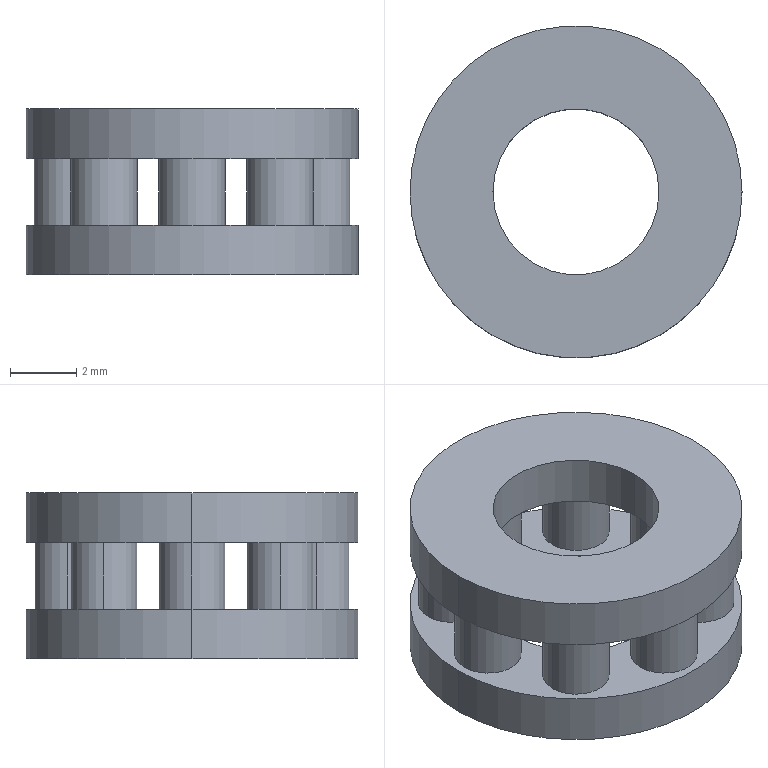Part | SolidWorks | features ICE 2, Extrusion 1 | 1 solid | 28 faces | box 10 x 10 x 5 mm | volume 226.98 mm3 | cylinder 24 | plane 4 | commonest cylinder face diameters 2 x16 5 x4 10 x4
STEP:
#1=CARTESIAN_POINT('',(-3.652,2.652,1.));
#2=VERTEX_POINT('',#1);
#3=CARTESIAN_POINT('',(-1.652,2.652,1.));
#4=VERTEX_POINT('',#3);
#5=CARTESIAN_POINT('',(-2.652,2.652,1.));
#6=DIRECTION('',(0.,0.,-1.));
#7=DIRECTION('',(1.,0.,0.));
#8=AXIS2_PLACEMENT_3D('',#5,#6,#7);
#9=CIRCLE('',#8,1.);
#10=EDGE_CURVE('',#2,#4,#9,.T.);
#11=ORIENTED_EDGE('',*,*,#10,.T.);
#12=CARTESIAN_POINT('',(-1.652,2.652,-1.));
#13=VERTEX_POINT('',#12);
#14=CARTESIAN_POINT('',(-1.652,2.652,1.));
#15=DIRECTION('',(0.,0.,-1.));
#16=VECTOR('',#15,1000.);
#17=LINE('',#14,#16);
#18=EDGE_CURVE('',#4,#13,#17,.T.);
#19=ORIENTED_EDGE('',*,*,#18,.T.);
#20=CARTESIAN_POINT('',(-3.652,2.652,-1.));
#21=VERTEX_POINT('',#20);
#22=CARTESIAN_POINT('',(-2.652,2.652,-1.));
#23=DIRECTION('',(0.,0.,1.));
#24=DIRECTION('',(1.,0.,0.));
#25=AXIS2_PLACEMENT_3D('',#22,#23,#24);
#26=CIRCLE('',#25,1.);
#27=EDGE_CURVE('',#13,#21,#26,.T.);
#28=ORIENTED_EDGE('',*,*,#27,.T.);
#29=CARTESIAN_POINT('',(-3.652,2.652,1.));
#30=DIRECTION('',(0.,0.,-1.));
#31=VECTOR('',#30,1000.);
#32=LINE('',#29,#31);
#33=EDGE_CURVE('',#2,#21,#32,.T.);
#34=ORIENTED_EDGE('',*,*,#33,.F.);
#35=EDGE_LOOP('',(#11,#19,#28,#34));
#36=FACE_OUTER_BOUND('',#35,.T.);
#37=CARTESIAN_POINT('',(-2.652,2.652,1.));
#38=DIRECTION('',(0.,0.,-1.));
#39=DIRECTION('',(-1.,0.,0.));
#40=AXIS2_PLACEMENT_3D('',#37,#38,#39);
#41=CYLINDRICAL_SURFACE('',#40,1.);
#42=ADVANCED_FACE('',(#36),#41,.T.);
#43=CARTESIAN_POINT('',(-4.75,0.,1.));
#44=VERTEX_POINT('',#43);
#45=CARTESIAN_POINT('',(-2.75,0.,1.));
#46=VERTEX_POINT('',#45);
#47=CARTESIAN_POINT('',(-3.75,0.,1.));
#48=DIRECTION('',(0.,0.,-1.));
#49=DIRECTION('',(1.,0.,0.));
#50=AXIS2_PLACEMENT_3D('',#47,#48,#49);
#51=CIRCLE('',#50,1.);
#52=EDGE_CURVE('',#44,#46,#51,.T.);
#53=ORIENTED_EDGE('',*,*,#52,.T.);
#54=CARTESIAN_POINT('',(-2.75,0.,-1.));
#55=VERTEX_POINT('',#54);
#56=CARTESIAN_POINT('',(-2.75,0.,1.));
#57=DIRECTION('',(0.,0.,-1.));
#58=VECTOR('',#57,1000.);
#59=LINE('',#56,#58);
#60=EDGE_CURVE('',#46,#55,#59,.T.);
#61=ORIENTED_EDGE('',*,*,#60,.T.);
#62=CARTESIAN_POINT('',(-4.75,0.,-1.));
#63=VERTEX_POINT('',#62);
#64=CARTESIAN_POINT('',(-3.75,0.,-1.));
#65=DIRECTION('',(0.,0.,1.));
#66=DIRECTION('',(1.,0.,0.));
#67=AXIS2_PLACEMENT_3D('',#64,#65,#66);
#68=CIRCLE('',#67,1.);
#69=EDGE_CURVE('',#55,#63,#68,.T.);
#70=ORIENTED_EDGE('',*,*,#69,.T.);
#71=CARTESIAN_POINT('',(-4.75,0.,1.));
#72=DIRECTION('',(0.,0.,-1.));
#73=VECTOR('',#72,1000.);
#74=LINE('',#71,#73);
#75=EDGE_CURVE('',#44,#63,#74,.T.);
#76=ORIENTED_EDGE('',*,*,#75,.F.);
#77=EDGE_LOOP('',(#53,#61,#70,#76));
#78=FACE_OUTER_BOUND('',#77,.T.);
#79=CARTESIAN_POINT('',(-3.75,0.,1.));
#80=DIRECTION('',(0.,0.,-1.));
#81=DIRECTION('',(-1.,0.,0.));
#82=AXIS2_PLACEMENT_3D('',#79,#80,#81);
#83=CYLINDRICAL_SURFACE('',#82,1.);
#84=ADVANCED_FACE('',(#78),#83,.T.);
#85=CARTESIAN_POINT('',(-3.652,-2.652,1.));
#86=VERTEX_POINT('',#85);
#87=CARTESIAN_POINT('',(-1.652,-2.652,1.));
#88=VERTEX_POINT('',#87);
#89=CARTESIAN_POINT('',(-2.652,-2.652,1.));
#90=DIRECTION('',(0.,0.,-1.));
#91=DIRECTION('',(1.,0.,0.));
#92=AXIS2_PLACEMENT_3D('',#89,#90,#91);
#93=CIRCLE('',#92,1.);
#94=EDGE_CURVE('',#86,#88,#93,.T.);
#95=ORIENTED_EDGE('',*,*,#94,.T.);
#96=CARTESIAN_POINT('',(-1.652,-2.652,-1.));
#97=VERTEX_POINT('',#96);
#98=CARTESIAN_POINT('',(-1.652,-2.652,1.));
#99=DIRECTION('',(0.,0.,-1.));
#100=VECTOR('',#99,1000.);
#101=LINE('',#98,#100);
#102=EDGE_CURVE('',#88,#97,#101,.T.);
#103=ORIENTED_EDGE('',*,*,#102,.T.);
#104=CARTESIAN_POINT('',(-3.652,-2.652,-1.));
#105=VERTEX_POINT('',#104);
#106=CARTESIAN_POINT('',(-2.652,-2.652,-1.));
#107=DIRECTION('',(0.,0.,1.));
#108=DIRECTION('',(1.,0.,0.));
#109=AXIS2_PLACEMENT_3D('',#106,#107,#108);
#110=CIRCLE('',#109,1.);
#111=EDGE_CURVE('',#97,#105,#110,.T.);
#112=ORIENTED_EDGE('',*,*,#111,.T.);
#113=CARTESIAN_POINT('',(-3.652,-2.652,1.));
#114=DIRECTION('',(0.,0.,-1.));
#115=VECTOR('',#114,1000.);
#116=LINE('',#113,#115);
#117=EDGE_CURVE('',#86,#105,#116,.T.);
#118=ORIENTED_EDGE('',*,*,#117,.F.);
#119=EDGE_LOOP('',(#95,#103,#112,#118));
#120=FACE_OUTER_BOUND('',#119,.T.);
#121=CARTESIAN_POINT('',(-2.652,-2.652,1.));
#122=DIRECTION('',(0.,0.,-1.));
#123=DIRECTION('',(-1.,0.,0.));
#124=AXIS2_PLACEMENT_3D('',#121,#122,#123);
#125=CYLINDRICAL_SURFACE('',#124,1.);
#126=ADVANCED_FACE('',(#120),#125,.T.);
#127=CARTESIAN_POINT('',(-1.,-3.75,1.));
#128=VERTEX_POINT('',#127);
#129=CARTESIAN_POINT('',(1.,-3.75,1.));
#130=VERTEX_POINT('',#129);
#131=CARTESIAN_POINT('',(0.,-3.75,1.));
#132=DIRECTION('',(0.,0.,-1.));
#133=DIRECTION('',(1.,0.,0.));
#134=AXIS2_PLACEMENT_3D('',#131,#132,#133);
#135=CIRCLE('',#134,1.);
#136=EDGE_CURVE('',#128,#130,#135,.T.);
#137=ORIENTED_EDGE('',*,*,#136,.T.);
#138=CARTESIAN_POINT('',(1.,-3.75,-1.));
#139=VERTEX_POINT('',#138);
#140=CARTESIAN_POINT('',(1.,-3.75,1.));
#141=DIRECTION('',(0.,0.,-1.));
#142=VECTOR('',#141,1000.);
#143=LINE('',#140,#142);
#144=EDGE_CURVE('',#130,#139,#143,.T.);
#145=ORIENTED_EDGE('',*,*,#144,.T.);
#146=CARTESIAN_POINT('',(-1.,-3.75,-1.));
#147=VERTEX_POINT('',#146);
#148=CARTESIAN_POINT('',(0.,-3.75,-1.));
#149=DIRECTION('',(0.,0.,1.));
#150=DIRECTION('',(1.,0.,0.));
#151=AXIS2_PLACEMENT_3D('',#148,#149,#150);
#152=CIRCLE('',#151,1.);
#153=EDGE_CURVE('',#139,#147,#152,.T.);
#154=ORIENTED_EDGE('',*,*,#153,.T.);
#155=CARTESIAN_POINT('',(-1.,-3.75,1.));
#156=DIRECTION('',(0.,0.,-1.));
#157=VECTOR('',#156,1000.);
#158=LINE('',#155,#157);
#159=EDGE_CURVE('',#128,#147,#158,.T.);
#160=ORIENTED_EDGE('',*,*,#159,.F.);
#161=EDGE_LOOP('',(#137,#145,#154,#160));
#162=FACE_OUTER_BOUND('',#161,.T.);
#163=CARTESIAN_POINT('',(0.,-3.75,1.));
#164=DIRECTION('',(0.,0.,-1.));
#165=DIRECTION('',(-1.,0.,0.));
#166=AXIS2_PLACEMENT_3D('',#163,#164,#165);
#167=CYLINDRICAL_SURFACE('',#166,1.);
#168=ADVANCED_FACE('',(#162),#167,.T.);
#169=CARTESIAN_POINT('',(1.652,-2.652,1.));
#170=VERTEX_POINT('',#169);
#171=CARTESIAN_POINT('',(3.652,-2.652,1.));
#172=VERTEX_POINT('',#171);
#173=CARTESIAN_POINT('',(2.652,-2.652,1.));
#174=DIRECTION('',(0.,0.,-1.));
#175=DIRECTION('',(1.,0.,0.));
#176=AXIS2_PLACEMENT_3D('',#173,#174,#175);
#177=CIRCLE('',#176,1.);
#178=EDGE_CURVE('',#170,#172,#177,.T.);
#179=ORIENTED_EDGE('',*,*,#178,.T.);
#180=CARTESIAN_POINT('',(3.652,-2.652,-1.));
#181=VERTEX_POINT('',#180);
#182=CARTESIAN_POINT('',(3.652,-2.652,1.));
#183=DIRECTION('',(0.,0.,-1.));
#184=VECTOR('',#183,1000.);
#185=LINE('',#182,#184);
#186=EDGE_CURVE('',#172,#181,#185,.T.);
#187=ORIENTED_EDGE('',*,*,#186,.T.);
#188=CARTESIAN_POINT('',(1.652,-2.652,-1.));
#189=VERTEX_POINT('',#188);
#190=CARTESIAN_POINT('',(2.652,-2.652,-1.));
#191=DIRECTION('',(0.,0.,1.));
#192=DIRECTION('',(1.,0.,0.));
#193=AXIS2_PLACEMENT_3D('',#190,#191,#192);
#194=CIRCLE('',#193,1.);
#195=EDGE_CURVE('',#181,#189,#194,.T.);
#196=ORIENTED_EDGE('',*,*,#195,.T.);
#197=CARTESIAN_POINT('',(1.652,-2.652,1.));
#198=DIRECTION('',(0.,0.,-1.));
#199=VECTOR('',#198,1000.);
#200=LINE('',#197,#199);
#201=EDGE_CURVE('',#170,#189,#200,.T.);
#202=ORIENTED_EDGE('',*,*,#201,.F.);
#203=EDGE_LOOP('',(#179,#187,#196,#202));
#204=FACE_OUTER_BOUND('',#203,.T.);
#205=CARTESIAN_POINT('',(2.652,-2.652,1.));
#206=DIRECTION('',(0.,0.,-1.));
#207=DIRECTION('',(-1.,0.,0.));
#208=AXIS2_PLACEMENT_3D('',#205,#206,#207);
#209=CYLINDRICAL_SURFACE('',#208,1.);
#210=ADVANCED_FACE('',(#204),#209,.T.);
#211=CARTESIAN_POINT('',(2.75,0.,1.));
#212=VERTEX_POINT('',#211);
#213=CARTESIAN_POINT('',(4.75,0.,1.));
#214=VERTEX_POINT('',#213);
#215=CARTESIAN_POINT('',(3.75,0.,1.));
#216=DIRECTION('',(0.,0.,-1.));
#217=DIRECTION('',(1.,0.,0.));
#218=AXIS2_PLACEMENT_3D('',#215,#216,#217);
#219=CIRCLE('',#218,1.);
#220=EDGE_CURVE('',#212,#214,#219,.T.);
#221=ORIENTED_EDGE('',*,*,#220,.T.);
#222=CARTESIAN_POINT('',(4.75,0.,-1.));
#223=VERTEX_POINT('',#222);
#224=CARTESIAN_POINT('',(4.75,0.,1.));
#225=DIRECTION('',(0.,0.,-1.));
#226=VECTOR('',#225,1000.);
#227=LINE('',#224,#226);
#228=EDGE_CURVE('',#214,#223,#227,.T.);
#229=ORIENTED_EDGE('',*,*,#228,.T.);
#230=CARTESIAN_POINT('',(2.75,0.,-1.));
#231=VERTEX_POINT('',#230);
#232=CARTESIAN_POINT('',(3.75,0.,-1.));
#233=DIRECTION('',(0.,0.,1.));
#234=DIRECTION('',(1.,0.,0.));
#235=AXIS2_PLACEMENT_3D('',#232,#233,#234);
#236=CIRCLE('',#235,1.);
#237=EDGE_CURVE('',#223,#231,#236,.T.);
#238=ORIENTED_EDGE('',*,*,#237,.T.);
#239=CARTESIAN_POINT('',(2.75,0.,1.));
#240=DIRECTION('',(0.,0.,-1.));
#241=VECTOR('',#240,1000.);
#242=LINE('',#239,#241);
#243=EDGE_CURVE('',#212,#231,#242,.T.);
#244=ORIENTED_EDGE('',*,*,#243,.F.);
#245=EDGE_LOOP('',(#221,#229,#238,#244));
#246=FACE_OUTER_BOUND('',#245,.T.);
#247=CARTESIAN_POINT('',(3.75,0.,1.));
#248=DIRECTION('',(0.,0.,-1.));
#249=DIRECTION('',(-1.,0.,0.));
#250=AXIS2_PLACEMENT_3D('',#247,#248,#249);
#251=CYLINDRICAL_SURFACE('',#250,1.);
#252=ADVANCED_FACE('',(#246),#251,.T.);
#253=CARTESIAN_POINT('',(1.652,2.652,1.));
#254=VERTEX_POINT('',#253);
#255=CARTESIAN_POINT('',(3.652,2.652,1.));
#256=VERTEX_POINT('',#255);
#257=CARTESIAN_POINT('',(2.652,2.652,1.));
#258=DIRECTION('',(0.,0.,-1.));
#259=DIRECTION('',(1.,0.,0.));
#260=AXIS2_PLACEMENT_3D('',#257,#258,#259);
#261=CIRCLE('',#260,1.);
#262=EDGE_CURVE('',#254,#256,#261,.T.);
#263=ORIENTED_EDGE('',*,*,#262,.T.);
#264=CARTESIAN_POINT('',(3.652,2.652,-1.));
#265=VERTEX_POINT('',#264);
#266=CARTESIAN_POINT('',(3.652,2.652,1.));
#267=DIRECTION('',(0.,0.,-1.));
#268=VECTOR('',#267,1000.);
#269=LINE('',#266,#268);
#270=EDGE_CURVE('',#256,#265,#269,.T.);
#271=ORIENTED_EDGE('',*,*,#270,.T.);
#272=CARTESIAN_POINT('',(1.652,2.652,-1.));
#273=VERTEX_POINT('',#272);
#274=CARTESIAN_POINT('',(2.652,2.652,-1.));
#275=DIRECTION('',(0.,0.,1.));
#276=DIRECTION('',(1.,0.,0.));
#277=AXIS2_PLACEMENT_3D('',#274,#275,#276);
#278=CIRCLE('',#277,1.);
#279=EDGE_CURVE('',#265,#273,#278,.T.);
#280=ORIENTED_EDGE('',*,*,#279,.T.);
#281=CARTESIAN_POINT('',(1.652,2.652,1.));
#282=DIRECTION('',(0.,0.,-1.));
#283=VECTOR('',#282,1000.);
#284=LINE('',#281,#283);
#285=EDGE_CURVE('',#254,#273,#284,.T.);
#286=ORIENTED_EDGE('',*,*,#285,.F.);
#287=EDGE_LOOP('',(#263,#271,#280,#286));
#288=FACE_OUTER_BOUND('',#287,.T.);
#289=CARTESIAN_POINT('',(2.652,2.652,1.));
#290=DIRECTION('',(0.,0.,-1.));
#291=DIRECTION('',(-1.,0.,0.));
#292=AXIS2_PLACEMENT_3D('',#289,#290,#291);
#293=CYLINDRICAL_SURFACE('',#292,1.);
#294=ADVANCED_FACE('',(#288),#293,.T.);
#295=CARTESIAN_POINT('',(-2.5,0.,-2.5));
#296=VERTEX_POINT('',#295);
#297=CARTESIAN_POINT('',(2.5,0.,-2.5));
#298=VERTEX_POINT('',#297);
#299=CARTESIAN_POINT('',(0.,0.,-2.5));
#300=DIRECTION('',(0.,0.,1.));
#301=DIRECTION('',(1.,0.,0.));
#302=AXIS2_PLACEMENT_3D('',#299,#300,#301);
#303=CIRCLE('',#302,2.5);
#304=EDGE_CURVE('',#296,#298,#303,.T.);
#305=ORIENTED_EDGE('',*,*,#304,.F.);
#306=CARTESIAN_POINT('',(-2.5,0.,-1.));
#307=VERTEX_POINT('',#306);
#308=CARTESIAN_POINT('',(-2.5,0.,-2.5));
#309=DIRECTION('',(0.,0.,1.));
#310=VECTOR('',#309,1000.);
#311=LINE('',#308,#310);
#312=EDGE_CURVE('',#296,#307,#311,.T.);
#313=ORIENTED_EDGE('',*,*,#312,.T.);
#314=CARTESIAN_POINT('',(2.5,0.,-1.));
#315=VERTEX_POINT('',#314);
#316=CARTESIAN_POINT('',(0.,0.,-1.));
#317=DIRECTION('',(0.,0.,1.));
#318=DIRECTION('',(1.,0.,0.));
#319=AXIS2_PLACEMENT_3D('',#316,#317,#318);
#320=CIRCLE('',#319,2.5);
#321=EDGE_CURVE('',#307,#315,#320,.T.);
#322=ORIENTED_EDGE('',*,*,#321,.T.);
#323=CARTESIAN_POINT('',(2.5,0.,-2.5));
#324=DIRECTION('',(0.,0.,1.));
#325=VECTOR('',#324,1000.);
#326=LINE('',#323,#325);
#327=EDGE_CURVE('',#298,#315,#326,.T.);
#328=ORIENTED_EDGE('',*,*,#327,.F.);
#329=EDGE_LOOP('',(#305,#313,#322,#328));
#330=FACE_OUTER_BOUND('',#329,.T.);
#331=CARTESIAN_POINT('',(0.,0.,-2.5));
#332=DIRECTION('',(0.,0.,1.));
#333=DIRECTION('',(1.,0.,0.));
#334=AXIS2_PLACEMENT_3D('',#331,#332,#333);
#335=CYLINDRICAL_SURFACE('',#334,2.5);
#336=ADVANCED_FACE('',(#330),#335,.F.);
#337=CARTESIAN_POINT('',(5.,0.,-2.5));
#338=VERTEX_POINT('',#337);
#339=CARTESIAN_POINT('',(-5.,0.,-2.5));
#340=VERTEX_POINT('',#339);
#341=CARTESIAN_POINT('',(0.,0.,-2.5));
#342=DIRECTION('',(0.,0.,1.));
#343=DIRECTION('',(1.,0.,0.));
#344=AXIS2_PLACEMENT_3D('',#341,#342,#343);
#345=CIRCLE('',#344,5.);
#346=EDGE_CURVE('',#338,#340,#345,.T.);
#347=ORIENTED_EDGE('',*,*,#346,.T.);
#348=CARTESIAN_POINT('',(-5.,0.,-1.));
#349=VERTEX_POINT('',#348);
#350=CARTESIAN_POINT('',(-5.,0.,-2.5));
#351=DIRECTION('',(0.,0.,1.));
#352=VECTOR('',#351,1000.);
#353=LINE('',#350,#352);
#354=EDGE_CURVE('',#340,#349,#353,.T.);
#355=ORIENTED_EDGE('',*,*,#354,.T.);
#356=CARTESIAN_POINT('',(5.,0.,-1.));
#357=VERTEX_POINT('',#356);
#358=CARTESIAN_POINT('',(0.,0.,-1.));
#359=DIRECTION('',(0.,0.,1.));
#360=DIRECTION('',(1.,0.,0.));
#361=AXIS2_PLACEMENT_3D('',#358,#359,#360);
#362=CIRCLE('',#361,5.);
#363=EDGE_CURVE('',#357,#349,#362,.T.);
#364=ORIENTED_EDGE('',*,*,#363,.F.);
#365=CARTESIAN_POINT('',(5.,0.,-2.5));
#366=DIRECTION('',(0.,0.,1.));
#367=VECTOR('',#366,1000.);
#368=LINE('',#365,#367);
#369=EDGE_CURVE('',#338,#357,#368,.T.);
#370=ORIENTED_EDGE('',*,*,#369,.F.);
#371=EDGE_LOOP('',(#347,#355,#364,#370));
#372=FACE_OUTER_BOUND('',#371,.T.);
#373=CARTESIAN_POINT('',(0.,0.,-2.5));
#374=DIRECTION('',(0.,0.,1.));
#375=DIRECTION('',(1.,0.,0.));
#376=AXIS2_PLACEMENT_3D('',#373,#374,#375);
#377=CYLINDRICAL_SURFACE('',#376,5.);
#378=ADVANCED_FACE('',(#372),#377,.T.);
#379=CARTESIAN_POINT('',(-1.,3.75,1.));
#380=VERTEX_POINT('',#379);
#381=CARTESIAN_POINT('',(1.,3.75,1.));
#382=VERTEX_POINT('',#381);
#383=CARTESIAN_POINT('',(0.,3.75,1.));
#384=DIRECTION('',(0.,0.,-1.));
#385=DIRECTION('',(1.,0.,0.));
#386=AXIS2_PLACEMENT_3D('',#383,#384,#385);
#387=CIRCLE('',#386,1.);
#388=EDGE_CURVE('',#380,#382,#387,.T.);
#389=ORIENTED_EDGE('',*,*,#388,.T.);
#390=CARTESIAN_POINT('',(1.,3.75,-1.));
#391=VERTEX_POINT('',#390);
#392=CARTESIAN_POINT('',(1.,3.75,1.));
#393=DIRECTION('',(0.,0.,-1.));
#394=VECTOR('',#393,1000.);
#395=LINE('',#392,#394);
#396=EDGE_CURVE('',#382,#391,#395,.T.);
#397=ORIENTED_EDGE('',*,*,#396,.T.);
#398=CARTESIAN_POINT('',(-1.,3.75,-1.));
#399=VERTEX_POINT('',#398);
#400=CARTESIAN_POINT('',(0.,3.75,-1.));
#401=DIRECTION('',(0.,0.,1.));
#402=DIRECTION('',(1.,0.,0.));
#403=AXIS2_PLACEMENT_3D('',#400,#401,#402);
#404=CIRCLE('',#403,1.);
#405=EDGE_CURVE('',#391,#399,#404,.T.);
#406=ORIENTED_EDGE('',*,*,#405,.T.);
#407=CARTESIAN_POINT('',(-1.,3.75,1.));
#408=DIRECTION('',(0.,0.,-1.));
#409=VECTOR('',#408,1000.);
#410=LINE('',#407,#409);
#411=EDGE_CURVE('',#380,#399,#410,.T.);
#412=ORIENTED_EDGE('',*,*,#411,.F.);
#413=EDGE_LOOP('',(#389,#397,#406,#412));
#414=FACE_OUTER_BOUND('',#413,.T.);
#415=CARTESIAN_POINT('',(0.,3.75,1.));
#416=DIRECTION('',(0.,0.,-1.));
#417=DIRECTION('',(-1.,0.,0.));
#418=AXIS2_PLACEMENT_3D('',#415,#416,#417);
#419=CYLINDRICAL_SURFACE('',#418,1.);
#420=ADVANCED_FACE('',(#414),#419,.T.);
#421=CARTESIAN_POINT('',(-2.5,0.,2.5));
#422=VERTEX_POINT('',#421);
#423=CARTESIAN_POINT('',(2.5,0.,2.5));
#424=VERTEX_POINT('',#423);
#425=CARTESIAN_POINT('',(0.,0.,2.5));
#426=DIRECTION('',(0.,0.,1.));
#427=DIRECTION('',(1.,0.,0.));
#428=AXIS2_PLACEMENT_3D('',#425,#426,#427);
#429=CIRCLE('',#428,2.5);
#430=EDGE_CURVE('',#422,#424,#429,.T.);
#431=ORIENTED_EDGE('',*,*,#430,.T.);
#432=CARTESIAN_POINT('',(2.5,0.,1.));
#433=VERTEX_POINT('',#432);
#434=CARTESIAN_POINT('',(2.5,0.,2.5));
#435=DIRECTION('',(0.,0.,-1.));
#436=VECTOR('',#435,1000.);
#437=LINE('',#434,#436);
#438=EDGE_CURVE('',#424,#433,#437,.T.);
#439=ORIENTED_EDGE('',*,*,#438,.T.);
#440=CARTESIAN_POINT('',(-2.5,0.,1.));
#441=VERTEX_POINT('',#440);
#442=CARTESIAN_POINT('',(0.,0.,1.));
#443=DIRECTION('',(0.,0.,1.));
#444=DIRECTION('',(1.,0.,0.));
#445=AXIS2_PLACEMENT_3D('',#442,#443,#444);
#446=CIRCLE('',#445,2.5);
#447=EDGE_CURVE('',#441,#433,#446,.T.);
#448=ORIENTED_EDGE('',*,*,#447,.F.);
#449=CARTESIAN_POINT('',(-2.5,0.,2.5));
#450=DIRECTION('',(0.,0.,-1.));
#451=VECTOR('',#450,1000.);
#452=LINE('',#449,#451);
#453=EDGE_CURVE('',#422,#441,#452,.T.);
#454=ORIENTED_EDGE('',*,*,#453,.F.);
#455=EDGE_LOOP('',(#431,#439,#448,#454));
#456=FACE_OUTER_BOUND('',#455,.T.);
#457=CARTESIAN_POINT('',(0.,0.,2.5));
#458=DIRECTION('',(0.,0.,-1.));
#459=DIRECTION('',(-1.,0.,0.));
#460=AXIS2_PLACEMENT_3D('',#457,#458,#459);
#461=CYLINDRICAL_SURFACE('',#460,2.5);
#462=ADVANCED_FACE('',(#456),#461,.F.);
#463=CARTESIAN_POINT('',(5.,0.,2.5));
#464=VERTEX_POINT('',#463);
#465=CARTESIAN_POINT('',(-5.,0.,2.5));
#466=VERTEX_POINT('',#465);
#467=CARTESIAN_POINT('',(0.,0.,2.5));
#468=DIRECTION('',(0.,0.,1.));
#469=DIRECTION('',(1.,0.,0.));
#470=AXIS2_PLACEMENT_3D('',#467,#468,#469);
#471=CIRCLE('',#470,5.);
#472=EDGE_CURVE('',#464,#466,#471,.T.);
#473=ORIENTED_EDGE('',*,*,#472,.F.);
#474=CARTESIAN_POINT('',(5.,0.,1.));
#475=VERTEX_POINT('',#474);
#476=CARTESIAN_POINT('',(5.,0.,2.5));
#477=DIRECTION('',(0.,0.,-1.));
#478=VECTOR('',#477,1000.);
#479=LINE('',#476,#478);
#480=EDGE_CURVE('',#464,#475,#479,.T.);
#481=ORIENTED_EDGE('',*,*,#480,.T.);
#482=CARTESIAN_POINT('',(-5.,0.,1.));
#483=VERTEX_POINT('',#482);
#484=CARTESIAN_POINT('',(0.,0.,1.));
#485=DIRECTION('',(0.,0.,1.));
#486=DIRECTION('',(1.,0.,0.));
#487=AXIS2_PLACEMENT_3D('',#484,#485,#486);
#488=CIRCLE('',#487,5.);
#489=EDGE_CURVE('',#475,#483,#488,.T.);
#490=ORIENTED_EDGE('',*,*,#489,.T.);
#491=CARTESIAN_POINT('',(-5.,0.,2.5));
#492=DIRECTION('',(0.,0.,-1.));
#493=VECTOR('',#492,1000.);
#494=LINE('',#491,#493);
#495=EDGE_CURVE('',#466,#483,#494,.T.);
#496=ORIENTED_EDGE('',*,*,#495,.F.);
#497=EDGE_LOOP('',(#473,#481,#490,#496));
#498=FACE_OUTER_BOUND('',#497,.T.);
#499=CARTESIAN_POINT('',(0.,0.,2.5));
#500=DIRECTION('',(0.,0.,-1.));
#501=DIRECTION('',(-1.,0.,0.));
#502=AXIS2_PLACEMENT_3D('',#499,#500,#501);
#503=CYLINDRICAL_SURFACE('',#502,5.);
#504=ADVANCED_FACE('',(#498),#503,.T.);
#505=CARTESIAN_POINT('',(0.,0.,2.5));
#506=DIRECTION('',(0.,0.,1.));
#507=DIRECTION('',(1.,0.,0.));
#508=AXIS2_PLACEMENT_3D('',#505,#506,#507);
#509=CIRCLE('',#508,5.);
#510=EDGE_CURVE('',#466,#464,#509,.T.);
#511=ORIENTED_EDGE('',*,*,#510,.T.);
#512=ORIENTED_EDGE('',*,*,#472,.T.);
#513=EDGE_LOOP('',(#511,#512));
#514=FACE_OUTER_BOUND('',#513,.T.);
#515=ORIENTED_EDGE('',*,*,#430,.F.);
#516=CARTESIAN_POINT('',(0.,0.,2.5));
#517=DIRECTION('',(0.,0.,1.));
#518=DIRECTION('',(1.,0.,0.));
#519=AXIS2_PLACEMENT_3D('',#516,#517,#518);
#520=CIRCLE('',#519,2.5);
#521=EDGE_CURVE('',#424,#422,#520,.T.);
#522=ORIENTED_EDGE('',*,*,#521,.F.);
#523=EDGE_LOOP('',(#515,#522));
#524=FACE_BOUND('',#523,.T.);
#525=CARTESIAN_POINT('',(0.,0.,2.5));
#526=DIRECTION('',(0.,0.,1.));
#527=DIRECTION('',(1.,0.,0.));
#528=AXIS2_PLACEMENT_3D('',#525,#526,#527);
#529=PLANE('',#528);
#530=ADVANCED_FACE('',(#514,#524),#529,.T.);
#531=ORIENTED_EDGE('',*,*,#10,.F.);
#532=CARTESIAN_POINT('',(-2.652,2.652,1.));
#533=DIRECTION('',(0.,0.,-1.));
#534=DIRECTION('',(1.,0.,0.));
#535=AXIS2_PLACEMENT_3D('',#532,#533,#534);
#536=CIRCLE('',#535,1.);
#537=EDGE_CURVE('',#4,#2,#536,.T.);
#538=ORIENTED_EDGE('',*,*,#537,.F.);
#539=EDGE_LOOP('',(#531,#538));
#540=FACE_BOUND('',#539,.T.);
#541=ORIENTED_EDGE('',*,*,#52,.F.);
#542=CARTESIAN_POINT('',(-3.75,0.,1.));
#543=DIRECTION('',(0.,0.,-1.));
#544=DIRECTION('',(1.,0.,0.));
#545=AXIS2_PLACEMENT_3D('',#542,#543,#544);
#546=CIRCLE('',#545,1.);
#547=EDGE_CURVE('',#46,#44,#546,.T.);
#548=ORIENTED_EDGE('',*,*,#547,.F.);
#549=EDGE_LOOP('',(#541,#548));
#550=FACE_BOUND('',#549,.T.);
#551=ORIENTED_EDGE('',*,*,#94,.F.);
#552=CARTESIAN_POINT('',(-2.652,-2.652,1.));
#553=DIRECTION('',(0.,0.,-1.));
#554=DIRECTION('',(1.,0.,0.));
#555=AXIS2_PLACEMENT_3D('',#552,#553,#554);
#556=CIRCLE('',#555,1.);
#557=EDGE_CURVE('',#88,#86,#556,.T.);
#558=ORIENTED_EDGE('',*,*,#557,.F.);
#559=EDGE_LOOP('',(#551,#558));
#560=FACE_BOUND('',#559,.T.);
#561=ORIENTED_EDGE('',*,*,#136,.F.);
#562=CARTESIAN_POINT('',(0.,-3.75,1.));
#563=DIRECTION('',(0.,0.,-1.));
#564=DIRECTION('',(1.,0.,0.));
#565=AXIS2_PLACEMENT_3D('',#562,#563,#564);
#566=CIRCLE('',#565,1.);
#567=EDGE_CURVE('',#130,#128,#566,.T.);
#568=ORIENTED_EDGE('',*,*,#567,.F.);
#569=EDGE_LOOP('',(#561,#568));
#570=FACE_BOUND('',#569,.T.);
#571=ORIENTED_EDGE('',*,*,#178,.F.);
#572=CARTESIAN_POINT('',(2.652,-2.652,1.));
#573=DIRECTION('',(0.,0.,-1.));
#574=DIRECTION('',(1.,0.,0.));
#575=AXIS2_PLACEMENT_3D('',#572,#573,#574);
#576=CIRCLE('',#575,1.);
#577=EDGE_CURVE('',#172,#170,#576,.T.);
#578=ORIENTED_EDGE('',*,*,#577,.F.);
#579=EDGE_LOOP('',(#571,#578));
#580=FACE_BOUND('',#579,.T.);
#581=ORIENTED_EDGE('',*,*,#220,.F.);
#582=CARTESIAN_POINT('',(3.75,0.,1.));
#583=DIRECTION('',(0.,0.,-1.));
#584=DIRECTION('',(1.,0.,0.));
#585=AXIS2_PLACEMENT_3D('',#582,#583,#584);
#586=CIRCLE('',#585,1.);
#587=EDGE_CURVE('',#214,#212,#586,.T.);
#588=ORIENTED_EDGE('',*,*,#587,.F.);
#589=EDGE_LOOP('',(#581,#588));
#590=FACE_BOUND('',#589,.T.);
#591=ORIENTED_EDGE('',*,*,#262,.F.);
#592=CARTESIAN_POINT('',(2.652,2.652,1.));
#593=DIRECTION('',(0.,0.,-1.));
#594=DIRECTION('',(1.,0.,0.));
#595=AXIS2_PLACEMENT_3D('',#592,#593,#594);
#596=CIRCLE('',#595,1.);
#597=EDGE_CURVE('',#256,#254,#596,.T.);
#598=ORIENTED_EDGE('',*,*,#597,.F.);
#599=EDGE_LOOP('',(#591,#598));
#600=FACE_BOUND('',#599,.T.);
#601=ORIENTED_EDGE('',*,*,#388,.F.);
#602=CARTESIAN_POINT('',(0.,3.75,1.));
#603=DIRECTION('',(0.,0.,-1.));
#604=DIRECTION('',(1.,0.,0.));
#605=AXIS2_PLACEMENT_3D('',#602,#603,#604);
#606=CIRCLE('',#605,1.);
#607=EDGE_CURVE('',#382,#380,#606,.T.);
#608=ORIENTED_EDGE('',*,*,#607,.F.);
#609=EDGE_LOOP('',(#601,#608));
#610=FACE_BOUND('',#609,.T.);
#611=CARTESIAN_POINT('',(0.,0.,1.));
#612=DIRECTION('',(0.,0.,1.));
#613=DIRECTION('',(1.,0.,0.));
#614=AXIS2_PLACEMENT_3D('',#611,#612,#613);
#615=CIRCLE('',#614,5.);
#616=EDGE_CURVE('',#483,#475,#615,.T.);
#617=ORIENTED_EDGE('',*,*,#616,.F.);
#618=ORIENTED_EDGE('',*,*,#489,.F.);
#619=EDGE_LOOP('',(#617,#618));
#620=FACE_OUTER_BOUND('',#619,.T.);
#621=ORIENTED_EDGE('',*,*,#447,.T.);
#622=CARTESIAN_POINT('',(0.,0.,1.));
#623=DIRECTION('',(0.,0.,1.));
#624=DIRECTION('',(1.,0.,0.));
#625=AXIS2_PLACEMENT_3D('',#622,#623,#624);
#626=CIRCLE('',#625,2.5);
#627=EDGE_CURVE('',#433,#441,#626,.T.);
#628=ORIENTED_EDGE('',*,*,#627,.T.);
#629=EDGE_LOOP('',(#621,#628));
#630=FACE_BOUND('',#629,.T.);
#631=CARTESIAN_POINT('',(0.,0.,1.));
#632=DIRECTION('',(0.,0.,1.));
#633=DIRECTION('',(1.,0.,0.));
#634=AXIS2_PLACEMENT_3D('',#631,#632,#633);
#635=PLANE('',#634);
#636=ADVANCED_FACE('',(#540,#550,#560,#570,#580,#590,#600,#610,#620,#630),#635,.F.);
#637=ORIENTED_EDGE('',*,*,#480,.F.);
#638=ORIENTED_EDGE('',*,*,#510,.F.);
#639=ORIENTED_EDGE('',*,*,#495,.T.);
#640=ORIENTED_EDGE('',*,*,#616,.T.);
#641=EDGE_LOOP('',(#637,#638,#639,#640));
#642=FACE_OUTER_BOUND('',#641,.T.);
#643=CARTESIAN_POINT('',(0.,0.,2.5));
#644=DIRECTION('',(0.,0.,-1.));
#645=DIRECTION('',(-1.,0.,0.));
#646=AXIS2_PLACEMENT_3D('',#643,#644,#645);
#647=CYLINDRICAL_SURFACE('',#646,5.);
#648=ADVANCED_FACE('',(#642),#647,.T.);
#649=ORIENTED_EDGE('',*,*,#438,.F.);
#650=ORIENTED_EDGE('',*,*,#521,.T.);
#651=ORIENTED_EDGE('',*,*,#453,.T.);
#652=ORIENTED_EDGE('',*,*,#627,.F.);
#653=EDGE_LOOP('',(#649,#650,#651,#652));
#654=FACE_OUTER_BOUND('',#653,.T.);
#655=CARTESIAN_POINT('',(0.,0.,2.5));
#656=DIRECTION('',(0.,0.,-1.));
#657=DIRECTION('',(-1.,0.,0.));
#658=AXIS2_PLACEMENT_3D('',#655,#656,#657);
#659=CYLINDRICAL_SURFACE('',#658,2.5);
#660=ADVANCED_FACE('',(#654),#659,.F.);
#661=ORIENTED_EDGE('',*,*,#396,.F.);
#662=ORIENTED_EDGE('',*,*,#607,.T.);
#663=ORIENTED_EDGE('',*,*,#411,.T.);
#664=CARTESIAN_POINT('',(0.,3.75,-1.));
#665=DIRECTION('',(0.,0.,1.));
#666=DIRECTION('',(1.,0.,0.));
#667=AXIS2_PLACEMENT_3D('',#664,#665,#666);
#668=CIRCLE('',#667,1.);
#669=EDGE_CURVE('',#399,#391,#668,.T.);
#670=ORIENTED_EDGE('',*,*,#669,.T.);
#671=EDGE_LOOP('',(#661,#662,#663,#670));
#672=FACE_OUTER_BOUND('',#671,.T.);
#673=CARTESIAN_POINT('',(0.,3.75,1.));
#674=DIRECTION('',(0.,0.,-1.));
#675=DIRECTION('',(-1.,0.,0.));
#676=AXIS2_PLACEMENT_3D('',#673,#674,#675);
#677=CYLINDRICAL_SURFACE('',#676,1.);
#678=ADVANCED_FACE('',(#672),#677,.T.);
#679=ORIENTED_EDGE('',*,*,#354,.F.);
#680=CARTESIAN_POINT('',(0.,0.,-2.5));
#681=DIRECTION('',(0.,0.,1.));
#682=DIRECTION('',(1.,0.,0.));
#683=AXIS2_PLACEMENT_3D('',#680,#681,#682);
#684=CIRCLE('',#683,5.);
#685=EDGE_CURVE('',#340,#338,#684,.T.);
#686=ORIENTED_EDGE('',*,*,#685,.T.);
#687=ORIENTED_EDGE('',*,*,#369,.T.);
#688=CARTESIAN_POINT('',(0.,0.,-1.));
#689=DIRECTION('',(0.,0.,1.));
#690=DIRECTION('',(1.,0.,0.));
#691=AXIS2_PLACEMENT_3D('',#688,#689,#690);
#692=CIRCLE('',#691,5.);
#693=EDGE_CURVE('',#349,#357,#692,.T.);
#694=ORIENTED_EDGE('',*,*,#693,.F.);
#695=EDGE_LOOP('',(#679,#686,#687,#694));
#696=FACE_OUTER_BOUND('',#695,.T.);
#697=CARTESIAN_POINT('',(0.,0.,-2.5));
#698=DIRECTION('',(0.,0.,1.));
#699=DIRECTION('',(1.,0.,0.));
#700=AXIS2_PLACEMENT_3D('',#697,#698,#699);
#701=CYLINDRICAL_SURFACE('',#700,5.);
#702=ADVANCED_FACE('',(#696),#701,.T.);
#703=CARTESIAN_POINT('',(0.,0.,-2.5));
#704=DIRECTION('',(0.,0.,1.));
#705=DIRECTION('',(1.,0.,0.));
#706=AXIS2_PLACEMENT_3D('',#703,#704,#705);
#707=CIRCLE('',#706,2.5);
#708=EDGE_CURVE('',#298,#296,#707,.T.);
#709=ORIENTED_EDGE('',*,*,#708,.T.);
#710=ORIENTED_EDGE('',*,*,#304,.T.);
#711=EDGE_LOOP('',(#709,#710));
#712=FACE_BOUND('',#711,.T.);
#713=ORIENTED_EDGE('',*,*,#346,.F.);
#714=ORIENTED_EDGE('',*,*,#685,.F.);
#715=EDGE_LOOP('',(#713,#714));
#716=FACE_OUTER_BOUND('',#715,.T.);
#717=CARTESIAN_POINT('',(0.,0.,-2.5));
#718=DIRECTION('',(0.,0.,1.));
#719=DIRECTION('',(1.,0.,0.));
#720=AXIS2_PLACEMENT_3D('',#717,#718,#719);
#721=PLANE('',#720);
#722=ADVANCED_FACE('',(#712,#716),#721,.F.);
#723=CARTESIAN_POINT('',(-2.652,2.652,-1.));
#724=DIRECTION('',(0.,0.,1.));
#725=DIRECTION('',(1.,0.,0.));
#726=AXIS2_PLACEMENT_3D('',#723,#724,#725);
#727=CIRCLE('',#726,1.);
#728=EDGE_CURVE('',#21,#13,#727,.T.);
#729=ORIENTED_EDGE('',*,*,#728,.F.);
#730=ORIENTED_EDGE('',*,*,#27,.F.);
#731=EDGE_LOOP('',(#729,#730));
#732=FACE_BOUND('',#731,.T.);
#733=CARTESIAN_POINT('',(-3.75,0.,-1.));
#734=DIRECTION('',(0.,0.,1.));
#735=DIRECTION('',(1.,0.,0.));
#736=AXIS2_PLACEMENT_3D('',#733,#734,#735);
#737=CIRCLE('',#736,1.);
#738=EDGE_CURVE('',#63,#55,#737,.T.);
#739=ORIENTED_EDGE('',*,*,#738,.F.);
#740=ORIENTED_EDGE('',*,*,#69,.F.);
#741=EDGE_LOOP('',(#739,#740));
#742=FACE_BOUND('',#741,.T.);
#743=CARTESIAN_POINT('',(-2.652,-2.652,-1.));
#744=DIRECTION('',(0.,0.,1.));
#745=DIRECTION('',(1.,0.,0.));
#746=AXIS2_PLACEMENT_3D('',#743,#744,#745);
#747=CIRCLE('',#746,1.);
#748=EDGE_CURVE('',#105,#97,#747,.T.);
#749=ORIENTED_EDGE('',*,*,#748,.F.);
#750=ORIENTED_EDGE('',*,*,#111,.F.);
#751=EDGE_LOOP('',(#749,#750));
#752=FACE_BOUND('',#751,.T.);
#753=CARTESIAN_POINT('',(0.,-3.75,-1.));
#754=DIRECTION('',(0.,0.,1.));
#755=DIRECTION('',(1.,0.,0.));
#756=AXIS2_PLACEMENT_3D('',#753,#754,#755);
#757=CIRCLE('',#756,1.);
#758=EDGE_CURVE('',#147,#139,#757,.T.);
#759=ORIENTED_EDGE('',*,*,#758,.F.);
#760=ORIENTED_EDGE('',*,*,#153,.F.);
#761=EDGE_LOOP('',(#759,#760));
#762=FACE_BOUND('',#761,.T.);
#763=CARTESIAN_POINT('',(2.652,-2.652,-1.));
#764=DIRECTION('',(0.,0.,1.));
#765=DIRECTION('',(1.,0.,0.));
#766=AXIS2_PLACEMENT_3D('',#763,#764,#765);
#767=CIRCLE('',#766,1.);
#768=EDGE_CURVE('',#189,#181,#767,.T.);
#769=ORIENTED_EDGE('',*,*,#768,.F.);
#770=ORIENTED_EDGE('',*,*,#195,.F.);
#771=EDGE_LOOP('',(#769,#770));
#772=FACE_BOUND('',#771,.T.);
#773=CARTESIAN_POINT('',(3.75,0.,-1.));
#774=DIRECTION('',(0.,0.,1.));
#775=DIRECTION('',(1.,0.,0.));
#776=AXIS2_PLACEMENT_3D('',#773,#774,#775);
#777=CIRCLE('',#776,1.);
#778=EDGE_CURVE('',#231,#223,#777,.T.);
#779=ORIENTED_EDGE('',*,*,#778,.F.);
#780=ORIENTED_EDGE('',*,*,#237,.F.);
#781=EDGE_LOOP('',(#779,#780));
#782=FACE_BOUND('',#781,.T.);
#783=CARTESIAN_POINT('',(2.652,2.652,-1.));
#784=DIRECTION('',(0.,0.,1.));
#785=DIRECTION('',(1.,0.,0.));
#786=AXIS2_PLACEMENT_3D('',#783,#784,#785);
#787=CIRCLE('',#786,1.);
#788=EDGE_CURVE('',#273,#265,#787,.T.);
#789=ORIENTED_EDGE('',*,*,#788,.F.);
#790=ORIENTED_EDGE('',*,*,#279,.F.);
#791=EDGE_LOOP('',(#789,#790));
#792=FACE_BOUND('',#791,.T.);
#793=ORIENTED_EDGE('',*,*,#669,.F.);
#794=ORIENTED_EDGE('',*,*,#405,.F.);
#795=EDGE_LOOP('',(#793,#794));
#796=FACE_BOUND('',#795,.T.);
#797=CARTESIAN_POINT('',(0.,0.,-1.));
#798=DIRECTION('',(0.,0.,1.));
#799=DIRECTION('',(1.,0.,0.));
#800=AXIS2_PLACEMENT_3D('',#797,#798,#799);
#801=CIRCLE('',#800,2.5);
#802=EDGE_CURVE('',#315,#307,#801,.T.);
#803=ORIENTED_EDGE('',*,*,#802,.F.);
#804=ORIENTED_EDGE('',*,*,#321,.F.);
#805=EDGE_LOOP('',(#803,#804));
#806=FACE_BOUND('',#805,.T.);
#807=ORIENTED_EDGE('',*,*,#363,.T.);
#808=ORIENTED_EDGE('',*,*,#693,.T.);
#809=EDGE_LOOP('',(#807,#808));
#810=FACE_OUTER_BOUND('',#809,.T.);
#811=CARTESIAN_POINT('',(0.,0.,-1.));
#812=DIRECTION('',(0.,0.,1.));
#813=DIRECTION('',(1.,0.,0.));
#814=AXIS2_PLACEMENT_3D('',#811,#812,#813);
#815=PLANE('',#814);
#816=ADVANCED_FACE('',(#732,#742,#752,#762,#772,#782,#792,#796,#806,#810),#815,.T.);
#817=ORIENTED_EDGE('',*,*,#312,.F.);
#818=ORIENTED_EDGE('',*,*,#708,.F.);
#819=ORIENTED_EDGE('',*,*,#327,.T.);
#820=ORIENTED_EDGE('',*,*,#802,.T.);
#821=EDGE_LOOP('',(#817,#818,#819,#820));
#822=FACE_OUTER_BOUND('',#821,.T.);
#823=CARTESIAN_POINT('',(0.,0.,-2.5));
#824=DIRECTION('',(0.,0.,1.));
#825=DIRECTION('',(1.,0.,0.));
#826=AXIS2_PLACEMENT_3D('',#823,#824,#825);
#827=CYLINDRICAL_SURFACE('',#826,2.5);
#828=ADVANCED_FACE('',(#822),#827,.F.);
#829=ORIENTED_EDGE('',*,*,#270,.F.);
#830=ORIENTED_EDGE('',*,*,#597,.T.);
#831=ORIENTED_EDGE('',*,*,#285,.T.);
#832=ORIENTED_EDGE('',*,*,#788,.T.);
#833=EDGE_LOOP('',(#829,#830,#831,#832));
#834=FACE_OUTER_BOUND('',#833,.T.);
#835=CARTESIAN_POINT('',(2.652,2.652,1.));
#836=DIRECTION('',(0.,0.,-1.));
#837=DIRECTION('',(-1.,0.,0.));
#838=AXIS2_PLACEMENT_3D('',#835,#836,#837);
#839=CYLINDRICAL_SURFACE('',#838,1.);
#840=ADVANCED_FACE('',(#834),#839,.T.);
#841=ORIENTED_EDGE('',*,*,#228,.F.);
#842=ORIENTED_EDGE('',*,*,#587,.T.);
#843=ORIENTED_EDGE('',*,*,#243,.T.);
#844=ORIENTED_EDGE('',*,*,#778,.T.);
#845=EDGE_LOOP('',(#841,#842,#843,#844));
#846=FACE_OUTER_BOUND('',#845,.T.);
#847=CARTESIAN_POINT('',(3.75,0.,1.));
#848=DIRECTION('',(0.,0.,-1.));
#849=DIRECTION('',(-1.,0.,0.));
#850=AXIS2_PLACEMENT_3D('',#847,#848,#849);
#851=CYLINDRICAL_SURFACE('',#850,1.);
#852=ADVANCED_FACE('',(#846),#851,.T.);
#853=ORIENTED_EDGE('',*,*,#186,.F.);
#854=ORIENTED_EDGE('',*,*,#577,.T.);
#855=ORIENTED_EDGE('',*,*,#201,.T.);
#856=ORIENTED_EDGE('',*,*,#768,.T.);
#857=EDGE_LOOP('',(#853,#854,#855,#856));
#858=FACE_OUTER_BOUND('',#857,.T.);
#859=CARTESIAN_POINT('',(2.652,-2.652,1.));
#860=DIRECTION('',(0.,0.,-1.));
#861=DIRECTION('',(-1.,0.,0.));
#862=AXIS2_PLACEMENT_3D('',#859,#860,#861);
#863=CYLINDRICAL_SURFACE('',#862,1.);
#864=ADVANCED_FACE('',(#858),#863,.T.);
#865=ORIENTED_EDGE('',*,*,#144,.F.);
#866=ORIENTED_EDGE('',*,*,#567,.T.);
#867=ORIENTED_EDGE('',*,*,#159,.T.);
#868=ORIENTED_EDGE('',*,*,#758,.T.);
#869=EDGE_LOOP('',(#865,#866,#867,#868));
#870=FACE_OUTER_BOUND('',#869,.T.);
#871=CARTESIAN_POINT('',(0.,-3.75,1.));
#872=DIRECTION('',(0.,0.,-1.));
#873=DIRECTION('',(-1.,0.,0.));
#874=AXIS2_PLACEMENT_3D('',#871,#872,#873);
#875=CYLINDRICAL_SURFACE('',#874,1.);
#876=ADVANCED_FACE('',(#870),#875,.T.);
#877=ORIENTED_EDGE('',*,*,#102,.F.);
#878=ORIENTED_EDGE('',*,*,#557,.T.);
#879=ORIENTED_EDGE('',*,*,#117,.T.);
#880=ORIENTED_EDGE('',*,*,#748,.T.);
#881=EDGE_LOOP('',(#877,#878,#879,#880));
#882=FACE_OUTER_BOUND('',#881,.T.);
#883=CARTESIAN_POINT('',(-2.652,-2.652,1.));
#884=DIRECTION('',(0.,0.,-1.));
#885=DIRECTION('',(-1.,0.,0.));
#886=AXIS2_PLACEMENT_3D('',#883,#884,#885);
#887=CYLINDRICAL_SURFACE('',#886,1.);
#888=ADVANCED_FACE('',(#882),#887,.T.);
#889=ORIENTED_EDGE('',*,*,#60,.F.);
#890=ORIENTED_EDGE('',*,*,#547,.T.);
#891=ORIENTED_EDGE('',*,*,#75,.T.);
#892=ORIENTED_EDGE('',*,*,#738,.T.);
#893=EDGE_LOOP('',(#889,#890,#891,#892));
#894=FACE_OUTER_BOUND('',#893,.T.);
#895=CARTESIAN_POINT('',(-3.75,0.,1.));
#896=DIRECTION('',(0.,0.,-1.));
#897=DIRECTION('',(-1.,0.,0.));
#898=AXIS2_PLACEMENT_3D('',#895,#896,#897);
#899=CYLINDRICAL_SURFACE('',#898,1.);
#900=ADVANCED_FACE('',(#894),#899,.T.);
#901=ORIENTED_EDGE('',*,*,#18,.F.);
#902=ORIENTED_EDGE('',*,*,#537,.T.);
#903=ORIENTED_EDGE('',*,*,#33,.T.);
#904=ORIENTED_EDGE('',*,*,#728,.T.);
#905=EDGE_LOOP('',(#901,#902,#903,#904));
#906=FACE_OUTER_BOUND('',#905,.T.);
#907=CARTESIAN_POINT('',(-2.652,2.652,1.));
#908=DIRECTION('',(0.,0.,-1.));
#909=DIRECTION('',(-1.,0.,0.));
#910=AXIS2_PLACEMENT_3D('',#907,#908,#909);
#911=CYLINDRICAL_SURFACE('',#910,1.);
#912=ADVANCED_FACE('',(#906),#911,.T.);
#913=CLOSED_SHELL('',(#42,#84,#126,#168,#210,#252,#294,#336,#378,#420,#462,#504,#530,#636,#648,#660,#678,#702,#722,#816,#828,#840,#852,#864,#876,#888,#900,#912));
#914=MANIFOLD_SOLID_BREP('',#913);
#915=CARTESIAN_POINT('',(0.,0.,0.));
#916=DIRECTION('',(0.,0.,1.));
#917=DIRECTION('',(1.,0.,0.));
#918=AXIS2_PLACEMENT_3D('',#915,#916,#917);
#919=(LENGTH_UNIT()NAMED_UNIT(*)SI_UNIT(.MILLI.,.METRE.));
#920=UNCERTAINTY_MEASURE_WITH_UNIT(LENGTH_MEASURE(0.00001),#919,'','');
#921=(NAMED_UNIT(*)PLANE_ANGLE_UNIT()SI_UNIT($,.RADIAN.));
#922=(NAMED_UNIT(*)SI_UNIT($,.STERADIAN.)SOLID_ANGLE_UNIT());
#923=(GEOMETRIC_REPRESENTATION_CONTEXT(3)GLOBAL_UNCERTAINTY_ASSIGNED_CONTEXT((#920))GLOBAL_UNIT_ASSIGNED_CONTEXT((#919,#921,#922))REPRESENTATION_CONTEXT('',''));
#924=ADVANCED_BREP_SHAPE_REPRESENTATION('',(#914,#918),#923);